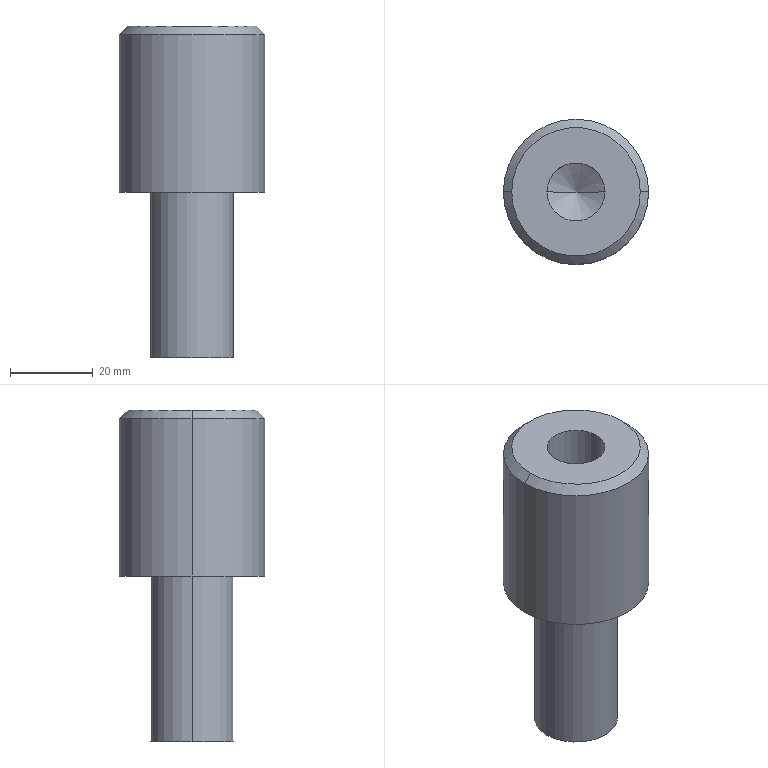Part | SolidWorks | features BaseBody 1 | 1 solid | 13 faces | box 35 x 35 x 80 mm | volume 47545 mm3 | cylinder 6 | cone 4 | plane 3 | commonest cylinder face diameters 14 x2 20 x2 35 x2
STEP:
#1=CARTESIAN_POINT('',(-17.5,0.,78.));
#2=VERTEX_POINT('',#1);
#3=CARTESIAN_POINT('',(17.5,0.,78.));
#4=VERTEX_POINT('',#3);
#5=CARTESIAN_POINT('',(0.,0.,78.));
#6=DIRECTION('',(0.,0.,-1.));
#7=DIRECTION('',(-1.,0.,0.));
#8=AXIS2_PLACEMENT_3D('',#5,#6,#7);
#9=CIRCLE('',#8,17.5);
#10=EDGE_CURVE('',#2,#4,#9,.T.);
#11=ORIENTED_EDGE('',*,*,#10,.T.);
#12=CARTESIAN_POINT('',(17.5,0.,40.));
#13=VERTEX_POINT('',#12);
#14=CARTESIAN_POINT('',(17.5,0.,80.));
#15=DIRECTION('',(0.,0.,-1.));
#16=VECTOR('',#15,1000.);
#17=LINE('',#14,#16);
#18=EDGE_CURVE('',#4,#13,#17,.T.);
#19=ORIENTED_EDGE('',*,*,#18,.T.);
#20=CARTESIAN_POINT('',(-17.5,0.,40.));
#21=VERTEX_POINT('',#20);
#22=CARTESIAN_POINT('',(0.,0.,40.));
#23=DIRECTION('',(0.,0.,1.));
#24=DIRECTION('',(-1.,0.,0.));
#25=AXIS2_PLACEMENT_3D('',#22,#23,#24);
#26=CIRCLE('',#25,17.5);
#27=EDGE_CURVE('',#13,#21,#26,.T.);
#28=ORIENTED_EDGE('',*,*,#27,.T.);
#29=CARTESIAN_POINT('',(-17.5,0.,80.));
#30=DIRECTION('',(0.,0.,-1.));
#31=VECTOR('',#30,1000.);
#32=LINE('',#29,#31);
#33=EDGE_CURVE('',#2,#21,#32,.T.);
#34=ORIENTED_EDGE('',*,*,#33,.F.);
#35=EDGE_LOOP('',(#11,#19,#28,#34));
#36=FACE_OUTER_BOUND('',#35,.T.);
#37=CARTESIAN_POINT('',(0.,0.,80.));
#38=DIRECTION('',(0.,0.,-1.));
#39=DIRECTION('',(-1.,0.,0.));
#40=AXIS2_PLACEMENT_3D('',#37,#38,#39);
#41=CYLINDRICAL_SURFACE('',#40,17.5);
#42=ADVANCED_FACE('',(#36),#41,.T.);
#43=CARTESIAN_POINT('',(-15.5,0.,80.));
#44=VERTEX_POINT('',#43);
#45=CARTESIAN_POINT('',(15.5,0.,80.));
#46=VERTEX_POINT('',#45);
#47=CARTESIAN_POINT('',(0.,0.,80.));
#48=DIRECTION('',(0.,0.,-1.));
#49=DIRECTION('',(-1.,0.,0.));
#50=AXIS2_PLACEMENT_3D('',#47,#48,#49);
#51=CIRCLE('',#50,15.5);
#52=EDGE_CURVE('',#44,#46,#51,.T.);
#53=ORIENTED_EDGE('',*,*,#52,.T.);
#54=CARTESIAN_POINT('',(17.5,0.,78.));
#55=DIRECTION('',(0.7071,0.,-0.7071));
#56=VECTOR('',#55,1000.);
#57=LINE('',#54,#56);
#58=EDGE_CURVE('',#46,#4,#57,.T.);
#59=ORIENTED_EDGE('',*,*,#58,.T.);
#60=ORIENTED_EDGE('',*,*,#10,.F.);
#61=CARTESIAN_POINT('',(-17.5,0.,78.));
#62=DIRECTION('',(-0.7071,0.,-0.7071));
#63=VECTOR('',#62,1000.);
#64=LINE('',#61,#63);
#65=EDGE_CURVE('',#44,#2,#64,.T.);
#66=ORIENTED_EDGE('',*,*,#65,.F.);
#67=EDGE_LOOP('',(#53,#59,#60,#66));
#68=FACE_OUTER_BOUND('',#67,.T.);
#69=CARTESIAN_POINT('',(0.,0.,78.));
#70=DIRECTION('',(0.,0.,-1.));
#71=DIRECTION('',(-1.,0.,0.));
#72=AXIS2_PLACEMENT_3D('',#69,#70,#71);
#73=CONICAL_SURFACE('',#72,17.5,0.7854);
#74=ADVANCED_FACE('',(#68),#73,.T.);
#75=CARTESIAN_POINT('',(-10.,0.,40.));
#76=VERTEX_POINT('',#75);
#77=CARTESIAN_POINT('',(10.,0.,40.));
#78=VERTEX_POINT('',#77);
#79=CARTESIAN_POINT('',(0.,0.,40.));
#80=DIRECTION('',(0.,0.,-1.));
#81=DIRECTION('',(-1.,0.,0.));
#82=AXIS2_PLACEMENT_3D('',#79,#80,#81);
#83=CIRCLE('',#82,10.);
#84=EDGE_CURVE('',#76,#78,#83,.T.);
#85=ORIENTED_EDGE('',*,*,#84,.T.);
#86=CARTESIAN_POINT('',(10.,0.,0.));
#87=VERTEX_POINT('',#86);
#88=CARTESIAN_POINT('',(10.,0.,40.));
#89=DIRECTION('',(0.,0.,-1.));
#90=VECTOR('',#89,1000.);
#91=LINE('',#88,#90);
#92=EDGE_CURVE('',#78,#87,#91,.T.);
#93=ORIENTED_EDGE('',*,*,#92,.T.);
#94=CARTESIAN_POINT('',(-10.,0.,0.));
#95=VERTEX_POINT('',#94);
#96=CARTESIAN_POINT('',(0.,0.,0.));
#97=DIRECTION('',(0.,0.,1.));
#98=DIRECTION('',(-1.,0.,0.));
#99=AXIS2_PLACEMENT_3D('',#96,#97,#98);
#100=CIRCLE('',#99,10.);
#101=EDGE_CURVE('',#87,#95,#100,.T.);
#102=ORIENTED_EDGE('',*,*,#101,.T.);
#103=CARTESIAN_POINT('',(-10.,0.,40.));
#104=DIRECTION('',(0.,0.,-1.));
#105=VECTOR('',#104,1000.);
#106=LINE('',#103,#105);
#107=EDGE_CURVE('',#76,#95,#106,.T.);
#108=ORIENTED_EDGE('',*,*,#107,.F.);
#109=EDGE_LOOP('',(#85,#93,#102,#108));
#110=FACE_OUTER_BOUND('',#109,.T.);
#111=CARTESIAN_POINT('',(0.,0.,40.));
#112=DIRECTION('',(0.,0.,-1.));
#113=DIRECTION('',(-1.,0.,0.));
#114=AXIS2_PLACEMENT_3D('',#111,#112,#113);
#115=CYLINDRICAL_SURFACE('',#114,10.);
#116=ADVANCED_FACE('',(#110),#115,.T.);
#117=CARTESIAN_POINT('',(-7.,0.,60.));
#118=VERTEX_POINT('',#117);
#119=CARTESIAN_POINT('',(7.,0.,60.));
#120=VERTEX_POINT('',#119);
#121=CARTESIAN_POINT('',(0.,0.,60.));
#122=DIRECTION('',(0.,0.,1.));
#123=DIRECTION('',(1.,0.,0.));
#124=AXIS2_PLACEMENT_3D('',#121,#122,#123);
#125=CIRCLE('',#124,7.);
#126=EDGE_CURVE('',#118,#120,#125,.T.);
#127=ORIENTED_EDGE('',*,*,#126,.F.);
#128=CARTESIAN_POINT('',(-7.,0.,80.));
#129=VERTEX_POINT('',#128);
#130=CARTESIAN_POINT('',(-7.,0.,80.));
#131=DIRECTION('',(0.,0.,1.));
#132=VECTOR('',#131,1000.);
#133=LINE('',#130,#132);
#134=EDGE_CURVE('',#118,#129,#133,.T.);
#135=ORIENTED_EDGE('',*,*,#134,.T.);
#136=CARTESIAN_POINT('',(7.,0.,80.));
#137=VERTEX_POINT('',#136);
#138=CARTESIAN_POINT('',(0.,0.,80.));
#139=DIRECTION('',(0.,0.,-1.));
#140=DIRECTION('',(1.,0.,0.));
#141=AXIS2_PLACEMENT_3D('',#138,#139,#140);
#142=CIRCLE('',#141,7.);
#143=EDGE_CURVE('',#137,#129,#142,.T.);
#144=ORIENTED_EDGE('',*,*,#143,.F.);
#145=CARTESIAN_POINT('',(7.,0.,80.));
#146=DIRECTION('',(0.,0.,1.));
#147=VECTOR('',#146,1000.);
#148=LINE('',#145,#147);
#149=EDGE_CURVE('',#120,#137,#148,.T.);
#150=ORIENTED_EDGE('',*,*,#149,.F.);
#151=EDGE_LOOP('',(#127,#135,#144,#150));
#152=FACE_OUTER_BOUND('',#151,.T.);
#153=CARTESIAN_POINT('',(0.,0.,80.));
#154=DIRECTION('',(0.,0.,1.));
#155=DIRECTION('',(1.,0.,0.));
#156=AXIS2_PLACEMENT_3D('',#153,#154,#155);
#157=CYLINDRICAL_SURFACE('',#156,7.);
#158=ADVANCED_FACE('',(#152),#157,.F.);
#159=CARTESIAN_POINT('',(0.,0.,55.794));
#160=VERTEX_POINT('',#159);
#161=CARTESIAN_POINT('',(7.,0.,60.));
#162=DIRECTION('',(0.8572,0.,0.515));
#163=VECTOR('',#162,1000.);
#164=LINE('',#161,#163);
#165=EDGE_CURVE('',#160,#120,#164,.T.);
#166=ORIENTED_EDGE('',*,*,#165,.F.);
#167=CARTESIAN_POINT('',(-7.,0.,60.));
#168=DIRECTION('',(-0.8572,0.,0.515));
#169=VECTOR('',#168,1000.);
#170=LINE('',#167,#169);
#171=EDGE_CURVE('',#160,#118,#170,.T.);
#172=ORIENTED_EDGE('',*,*,#171,.T.);
#173=ORIENTED_EDGE('',*,*,#126,.T.);
#174=EDGE_LOOP('',(#166,#172,#173));
#175=FACE_OUTER_BOUND('',#174,.T.);
#176=CARTESIAN_POINT('',(0.,0.,60.));
#177=DIRECTION('',(0.,0.,1.));
#178=DIRECTION('',(1.,0.,0.));
#179=AXIS2_PLACEMENT_3D('',#176,#177,#178);
#180=CONICAL_SURFACE('',#179,7.,1.03);
#181=ADVANCED_FACE('',(#175),#180,.F.);
#182=ORIENTED_EDGE('',*,*,#18,.F.);
#183=CARTESIAN_POINT('',(0.,0.,78.));
#184=DIRECTION('',(0.,0.,-1.));
#185=DIRECTION('',(-1.,0.,0.));
#186=AXIS2_PLACEMENT_3D('',#183,#184,#185);
#187=CIRCLE('',#186,17.5);
#188=EDGE_CURVE('',#4,#2,#187,.T.);
#189=ORIENTED_EDGE('',*,*,#188,.T.);
#190=ORIENTED_EDGE('',*,*,#33,.T.);
#191=CARTESIAN_POINT('',(0.,0.,40.));
#192=DIRECTION('',(0.,0.,1.));
#193=DIRECTION('',(-1.,0.,0.));
#194=AXIS2_PLACEMENT_3D('',#191,#192,#193);
#195=CIRCLE('',#194,17.5);
#196=EDGE_CURVE('',#21,#13,#195,.T.);
#197=ORIENTED_EDGE('',*,*,#196,.T.);
#198=EDGE_LOOP('',(#182,#189,#190,#197));
#199=FACE_OUTER_BOUND('',#198,.T.);
#200=CARTESIAN_POINT('',(0.,0.,80.));
#201=DIRECTION('',(0.,0.,-1.));
#202=DIRECTION('',(-1.,0.,0.));
#203=AXIS2_PLACEMENT_3D('',#200,#201,#202);
#204=CYLINDRICAL_SURFACE('',#203,17.5);
#205=ADVANCED_FACE('',(#199),#204,.T.);
#206=ORIENTED_EDGE('',*,*,#196,.F.);
#207=ORIENTED_EDGE('',*,*,#27,.F.);
#208=EDGE_LOOP('',(#206,#207));
#209=FACE_OUTER_BOUND('',#208,.T.);
#210=ORIENTED_EDGE('',*,*,#84,.F.);
#211=CARTESIAN_POINT('',(0.,0.,40.));
#212=DIRECTION('',(0.,0.,-1.));
#213=DIRECTION('',(-1.,0.,0.));
#214=AXIS2_PLACEMENT_3D('',#211,#212,#213);
#215=CIRCLE('',#214,10.);
#216=EDGE_CURVE('',#78,#76,#215,.T.);
#217=ORIENTED_EDGE('',*,*,#216,.F.);
#218=EDGE_LOOP('',(#210,#217));
#219=FACE_BOUND('',#218,.T.);
#220=CARTESIAN_POINT('',(0.,0.,40.));
#221=DIRECTION('',(0.,0.,1.));
#222=DIRECTION('',(1.,0.,0.));
#223=AXIS2_PLACEMENT_3D('',#220,#221,#222);
#224=PLANE('',#223);
#225=ADVANCED_FACE('',(#209,#219),#224,.F.);
#226=ORIENTED_EDGE('',*,*,#58,.F.);
#227=CARTESIAN_POINT('',(0.,0.,80.));
#228=DIRECTION('',(0.,0.,-1.));
#229=DIRECTION('',(-1.,0.,0.));
#230=AXIS2_PLACEMENT_3D('',#227,#228,#229);
#231=CIRCLE('',#230,15.5);
#232=EDGE_CURVE('',#46,#44,#231,.T.);
#233=ORIENTED_EDGE('',*,*,#232,.T.);
#234=ORIENTED_EDGE('',*,*,#65,.T.);
#235=ORIENTED_EDGE('',*,*,#188,.F.);
#236=EDGE_LOOP('',(#226,#233,#234,#235));
#237=FACE_OUTER_BOUND('',#236,.T.);
#238=CARTESIAN_POINT('',(0.,0.,78.));
#239=DIRECTION('',(0.,0.,-1.));
#240=DIRECTION('',(-1.,0.,0.));
#241=AXIS2_PLACEMENT_3D('',#238,#239,#240);
#242=CONICAL_SURFACE('',#241,17.5,0.7854);
#243=ADVANCED_FACE('',(#237),#242,.T.);
#244=ORIENTED_EDGE('',*,*,#92,.F.);
#245=ORIENTED_EDGE('',*,*,#216,.T.);
#246=ORIENTED_EDGE('',*,*,#107,.T.);
#247=CARTESIAN_POINT('',(0.,0.,0.));
#248=DIRECTION('',(0.,0.,1.));
#249=DIRECTION('',(-1.,0.,0.));
#250=AXIS2_PLACEMENT_3D('',#247,#248,#249);
#251=CIRCLE('',#250,10.);
#252=EDGE_CURVE('',#95,#87,#251,.T.);
#253=ORIENTED_EDGE('',*,*,#252,.T.);
#254=EDGE_LOOP('',(#244,#245,#246,#253));
#255=FACE_OUTER_BOUND('',#254,.T.);
#256=CARTESIAN_POINT('',(0.,0.,40.));
#257=DIRECTION('',(0.,0.,-1.));
#258=DIRECTION('',(-1.,0.,0.));
#259=AXIS2_PLACEMENT_3D('',#256,#257,#258);
#260=CYLINDRICAL_SURFACE('',#259,10.);
#261=ADVANCED_FACE('',(#255),#260,.T.);
#262=ORIENTED_EDGE('',*,*,#143,.T.);
#263=CARTESIAN_POINT('',(0.,0.,80.));
#264=DIRECTION('',(0.,0.,-1.));
#265=DIRECTION('',(1.,0.,0.));
#266=AXIS2_PLACEMENT_3D('',#263,#264,#265);
#267=CIRCLE('',#266,7.);
#268=EDGE_CURVE('',#129,#137,#267,.T.);
#269=ORIENTED_EDGE('',*,*,#268,.T.);
#270=EDGE_LOOP('',(#262,#269));
#271=FACE_BOUND('',#270,.T.);
#272=ORIENTED_EDGE('',*,*,#52,.F.);
#273=ORIENTED_EDGE('',*,*,#232,.F.);
#274=EDGE_LOOP('',(#272,#273));
#275=FACE_OUTER_BOUND('',#274,.T.);
#276=CARTESIAN_POINT('',(0.,0.,80.));
#277=DIRECTION('',(0.,0.,1.));
#278=DIRECTION('',(1.,0.,0.));
#279=AXIS2_PLACEMENT_3D('',#276,#277,#278);
#280=PLANE('',#279);
#281=ADVANCED_FACE('',(#271,#275),#280,.T.);
#282=ORIENTED_EDGE('',*,*,#252,.F.);
#283=ORIENTED_EDGE('',*,*,#101,.F.);
#284=EDGE_LOOP('',(#282,#283));
#285=FACE_OUTER_BOUND('',#284,.T.);
#286=CARTESIAN_POINT('',(0.,0.,0.));
#287=DIRECTION('',(0.,0.,1.));
#288=DIRECTION('',(1.,0.,0.));
#289=AXIS2_PLACEMENT_3D('',#286,#287,#288);
#290=PLANE('',#289);
#291=ADVANCED_FACE('',(#285),#290,.F.);
#292=ORIENTED_EDGE('',*,*,#134,.F.);
#293=CARTESIAN_POINT('',(0.,0.,60.));
#294=DIRECTION('',(0.,0.,1.));
#295=DIRECTION('',(1.,0.,0.));
#296=AXIS2_PLACEMENT_3D('',#293,#294,#295);
#297=CIRCLE('',#296,7.);
#298=EDGE_CURVE('',#120,#118,#297,.T.);
#299=ORIENTED_EDGE('',*,*,#298,.F.);
#300=ORIENTED_EDGE('',*,*,#149,.T.);
#301=ORIENTED_EDGE('',*,*,#268,.F.);
#302=EDGE_LOOP('',(#292,#299,#300,#301));
#303=FACE_OUTER_BOUND('',#302,.T.);
#304=CARTESIAN_POINT('',(0.,0.,80.));
#305=DIRECTION('',(0.,0.,1.));
#306=DIRECTION('',(1.,0.,0.));
#307=AXIS2_PLACEMENT_3D('',#304,#305,#306);
#308=CYLINDRICAL_SURFACE('',#307,7.);
#309=ADVANCED_FACE('',(#303),#308,.F.);
#310=ORIENTED_EDGE('',*,*,#171,.F.);
#311=ORIENTED_EDGE('',*,*,#165,.T.);
#312=ORIENTED_EDGE('',*,*,#298,.T.);
#313=EDGE_LOOP('',(#310,#311,#312));
#314=FACE_OUTER_BOUND('',#313,.T.);
#315=CARTESIAN_POINT('',(0.,0.,60.));
#316=DIRECTION('',(0.,0.,1.));
#317=DIRECTION('',(1.,0.,0.));
#318=AXIS2_PLACEMENT_3D('',#315,#316,#317);
#319=CONICAL_SURFACE('',#318,7.,1.03);
#320=ADVANCED_FACE('',(#314),#319,.F.);
#321=CLOSED_SHELL('',(#42,#74,#116,#158,#181,#205,#225,#243,#261,#281,#291,#309,#320));
#322=MANIFOLD_SOLID_BREP('',#321);
#323=CARTESIAN_POINT('',(0.,0.,0.));
#324=DIRECTION('',(0.,0.,1.));
#325=DIRECTION('',(1.,0.,0.));
#326=AXIS2_PLACEMENT_3D('',#323,#324,#325);
#327=(LENGTH_UNIT()NAMED_UNIT(*)SI_UNIT(.MILLI.,.METRE.));
#328=UNCERTAINTY_MEASURE_WITH_UNIT(LENGTH_MEASURE(0.00001),#327,'','');
#329=(NAMED_UNIT(*)PLANE_ANGLE_UNIT()SI_UNIT($,.RADIAN.));
#330=(NAMED_UNIT(*)SI_UNIT($,.STERADIAN.)SOLID_ANGLE_UNIT());
#331=(GEOMETRIC_REPRESENTATION_CONTEXT(3)GLOBAL_UNCERTAINTY_ASSIGNED_CONTEXT((#328))GLOBAL_UNIT_ASSIGNED_CONTEXT((#327,#329,#330))REPRESENTATION_CONTEXT('',''));
#332=ADVANCED_BREP_SHAPE_REPRESENTATION('',(#322,#326),#331);